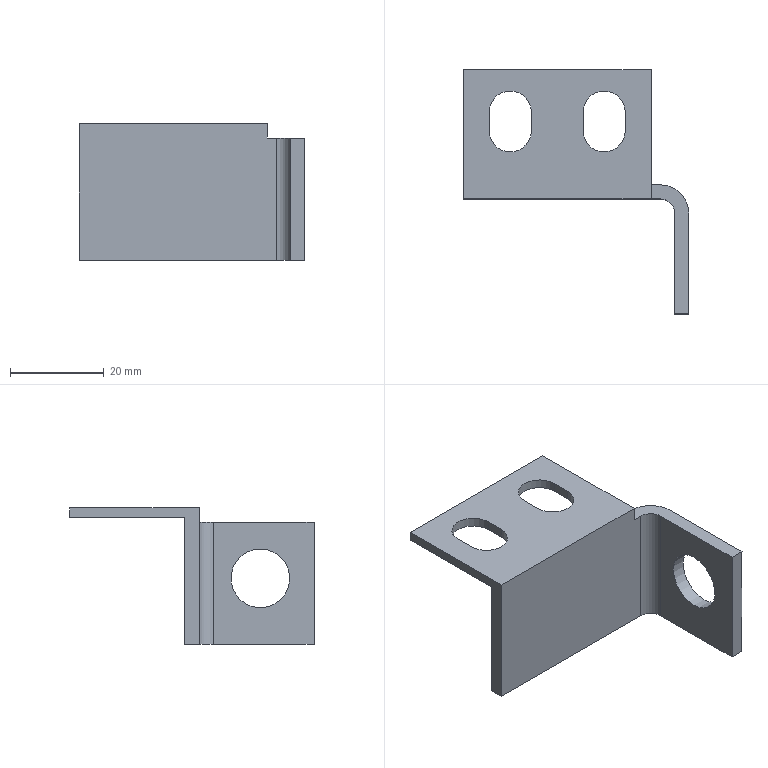Part | STEP file | lll_id4786_x_t | 1 solid | 23 faces | box 48 x 52 x 29 mm | volume 7058 mm3 | plane 16 | cylinder 7 | commonest cylinder face diameters 9 x4 6 x1 12 x1 12.5 x1
STEP:
#1=CARTESIAN_POINT('',(714.278,-390.043,-0.00000003));
#2=VERTEX_POINT('',#1);
#3=CARTESIAN_POINT('',(705.278,-390.043,-0.00000003));
#4=VERTEX_POINT('',#3);
#5=CARTESIAN_POINT('',(709.778,-390.043,-0.00000003));
#6=DIRECTION('',(0.,0.,1.));
#7=DIRECTION('',(1.,0.,0.));
#8=AXIS2_PLACEMENT_3D('',#5,#6,#7);
#9=CIRCLE('',#8,4.5);
#10=EDGE_CURVE('',#2,#4,#9,.T.);
#11=ORIENTED_EDGE('',*,*,#10,.T.);
#12=CARTESIAN_POINT('',(705.278,-394.043,-0.00000003));
#13=VERTEX_POINT('',#12);
#14=CARTESIAN_POINT('',(705.278,-392.043,-0.00000003));
#15=DIRECTION('',(0.,-1.,0.));
#16=VECTOR('',#15,1.);
#17=LINE('',#14,#16);
#18=EDGE_CURVE('',#4,#13,#17,.T.);
#19=ORIENTED_EDGE('',*,*,#18,.T.);
#20=CARTESIAN_POINT('',(714.278,-394.043,-0.00000003));
#21=VERTEX_POINT('',#20);
#22=CARTESIAN_POINT('',(709.778,-394.043,0.000000001));
#23=DIRECTION('',(0.,0.,-1.));
#24=DIRECTION('',(1.,0.,0.));
#25=AXIS2_PLACEMENT_3D('',#22,#23,#24);
#26=CIRCLE('',#25,4.5);
#27=EDGE_CURVE('',#21,#13,#26,.T.);
#28=ORIENTED_EDGE('',*,*,#27,.F.);
#29=CARTESIAN_POINT('',(714.278,-392.043,-0.00000003));
#30=DIRECTION('',(0.,1.,0.));
#31=VECTOR('',#30,1.);
#32=LINE('',#29,#31);
#33=EDGE_CURVE('',#21,#2,#32,.T.);
#34=ORIENTED_EDGE('',*,*,#33,.T.);
#35=EDGE_LOOP('',(#11,#19,#28,#34));
#36=FACE_BOUND('',#35,.T.);
#37=CARTESIAN_POINT('',(699.778,-405.543,0.000000001));
#38=VERTEX_POINT('',#37);
#39=CARTESIAN_POINT('',(739.778,-405.543,0.));
#40=VERTEX_POINT('',#39);
#41=CARTESIAN_POINT('',(758.537,-405.543,-0.000000001));
#42=DIRECTION('',(1.,0.,0.));
#43=VECTOR('',#42,1.);
#44=LINE('',#41,#43);
#45=EDGE_CURVE('',#38,#40,#44,.T.);
#46=ORIENTED_EDGE('',*,*,#45,.F.);
#47=CARTESIAN_POINT('',(699.778,-381.043,0.000000001));
#48=VERTEX_POINT('',#47);
#49=CARTESIAN_POINT('',(699.778,-172.043,0.000000001));
#50=DIRECTION('',(0.,1.,0.));
#51=VECTOR('',#50,1.);
#52=LINE('',#49,#51);
#53=EDGE_CURVE('',#38,#48,#52,.T.);
#54=ORIENTED_EDGE('',*,*,#53,.T.);
#55=CARTESIAN_POINT('',(739.778,-381.043,0.));
#56=VERTEX_POINT('',#55);
#57=CARTESIAN_POINT('',(1322.642,-381.043,-0.000000019));
#58=DIRECTION('',(1.,0.,0.));
#59=VECTOR('',#58,1.);
#60=LINE('',#57,#59);
#61=EDGE_CURVE('',#48,#56,#60,.T.);
#62=ORIENTED_EDGE('',*,*,#61,.T.);
#63=CARTESIAN_POINT('',(739.778,-397.043,0.));
#64=DIRECTION('',(0.,-1.,0.));
#65=VECTOR('',#64,1.);
#66=LINE('',#63,#65);
#67=EDGE_CURVE('',#56,#40,#66,.T.);
#68=ORIENTED_EDGE('',*,*,#67,.T.);
#69=EDGE_LOOP('',(#46,#54,#62,#68));
#70=FACE_BOUND('',#69,.T.);
#71=CARTESIAN_POINT('',(725.278,-390.043,-0.00000003));
#72=VERTEX_POINT('',#71);
#73=CARTESIAN_POINT('',(734.278,-390.043,-0.00000003));
#74=VERTEX_POINT('',#73);
#75=CARTESIAN_POINT('',(729.778,-390.043,-0.00000003));
#76=DIRECTION('',(0.,0.,-1.));
#77=DIRECTION('',(-1.,0.,0.));
#78=AXIS2_PLACEMENT_3D('',#75,#76,#77);
#79=CIRCLE('',#78,4.5);
#80=EDGE_CURVE('',#72,#74,#79,.T.);
#81=ORIENTED_EDGE('',*,*,#80,.F.);
#82=CARTESIAN_POINT('',(725.278,-394.043,-0.00000003));
#83=VERTEX_POINT('',#82);
#84=CARTESIAN_POINT('',(725.278,-392.043,-0.00000003));
#85=DIRECTION('',(0.,-1.,0.));
#86=VECTOR('',#85,1.);
#87=LINE('',#84,#86);
#88=EDGE_CURVE('',#72,#83,#87,.T.);
#89=ORIENTED_EDGE('',*,*,#88,.T.);
#90=CARTESIAN_POINT('',(734.278,-394.043,-0.00000003));
#91=VERTEX_POINT('',#90);
#92=CARTESIAN_POINT('',(729.778,-394.043,0.));
#93=DIRECTION('',(0.,0.,-1.));
#94=DIRECTION('',(-1.,0.,0.));
#95=AXIS2_PLACEMENT_3D('',#92,#93,#94);
#96=CIRCLE('',#95,4.5);
#97=EDGE_CURVE('',#91,#83,#96,.T.);
#98=ORIENTED_EDGE('',*,*,#97,.F.);
#99=CARTESIAN_POINT('',(734.278,-392.043,-0.00000003));
#100=DIRECTION('',(0.,1.,0.));
#101=VECTOR('',#100,1.);
#102=LINE('',#99,#101);
#103=EDGE_CURVE('',#91,#74,#102,.T.);
#104=ORIENTED_EDGE('',*,*,#103,.T.);
#105=EDGE_LOOP('',(#81,#89,#98,#104));
#106=FACE_BOUND('',#105,.T.);
#107=CARTESIAN_POINT('',(758.537,-172.043,-0.000000001));
#108=DIRECTION('',(0.,0.,-1.));
#109=DIRECTION('',(-1.,0.,0.));
#110=AXIS2_PLACEMENT_3D('',#107,#108,#109);
#111=PLANE('',#110);
#112=ADVANCED_FACE('',(#36,#70,#106),#111,.T.);
#113=CARTESIAN_POINT('',(739.778,-408.543,-1.));
#114=VERTEX_POINT('',#113);
#115=CARTESIAN_POINT('',(741.778,-408.543,-1.));
#116=VERTEX_POINT('',#115);
#117=CARTESIAN_POINT('',(712.778,-408.543,-1.));
#118=DIRECTION('',(1.,0.,0.));
#119=VECTOR('',#118,1.);
#120=LINE('',#117,#119);
#121=EDGE_CURVE('',#114,#116,#120,.T.);
#122=ORIENTED_EDGE('',*,*,#121,.F.);
#123=CARTESIAN_POINT('',(739.778,-408.543,2.));
#124=VERTEX_POINT('',#123);
#125=CARTESIAN_POINT('',(739.778,-408.543,-50.5));
#126=DIRECTION('',(0.,0.,1.));
#127=VECTOR('',#126,1.);
#128=LINE('',#125,#127);
#129=EDGE_CURVE('',#114,#124,#128,.T.);
#130=ORIENTED_EDGE('',*,*,#129,.T.);
#131=CARTESIAN_POINT('',(699.778,-408.543,2.));
#132=VERTEX_POINT('',#131);
#133=CARTESIAN_POINT('',(712.778,-408.543,2.));
#134=DIRECTION('',(1.,0.,0.));
#135=VECTOR('',#134,1.);
#136=LINE('',#133,#135);
#137=EDGE_CURVE('',#132,#124,#136,.T.);
#138=ORIENTED_EDGE('',*,*,#137,.F.);
#139=CARTESIAN_POINT('',(699.778,-408.543,-27.));
#140=VERTEX_POINT('',#139);
#141=CARTESIAN_POINT('',(699.778,-408.543,-50.5));
#142=DIRECTION('',(0.,0.,1.));
#143=VECTOR('',#142,1.);
#144=LINE('',#141,#143);
#145=EDGE_CURVE('',#140,#132,#144,.T.);
#146=ORIENTED_EDGE('',*,*,#145,.F.);
#147=CARTESIAN_POINT('',(741.778,-408.543,-27.));
#148=VERTEX_POINT('',#147);
#149=CARTESIAN_POINT('',(712.778,-408.543,-27.));
#150=DIRECTION('',(1.,0.,0.));
#151=VECTOR('',#150,1.);
#152=LINE('',#149,#151);
#153=EDGE_CURVE('',#140,#148,#152,.T.);
#154=ORIENTED_EDGE('',*,*,#153,.T.);
#155=CARTESIAN_POINT('',(741.778,-408.543,-55.5));
#156=DIRECTION('',(0.,0.,-1.));
#157=VECTOR('',#156,1.);
#158=LINE('',#155,#157);
#159=EDGE_CURVE('',#116,#148,#158,.T.);
#160=ORIENTED_EDGE('',*,*,#159,.F.);
#161=EDGE_LOOP('',(#122,#130,#138,#146,#154,#160));
#162=FACE_OUTER_BOUND('',#161,.T.);
#163=CARTESIAN_POINT('',(712.778,-408.543,-55.5));
#164=DIRECTION('',(0.,-1.,0.));
#165=DIRECTION('',(0.,0.,1.));
#166=AXIS2_PLACEMENT_3D('',#163,#164,#165);
#167=PLANE('',#166);
#168=ADVANCED_FACE('',(#162),#167,.T.);
#169=CARTESIAN_POINT('',(699.778,-405.543,-27.));
#170=VERTEX_POINT('',#169);
#171=CARTESIAN_POINT('',(741.778,-405.543,-27.));
#172=VERTEX_POINT('',#171);
#173=CARTESIAN_POINT('',(656.912,-405.543,-27.));
#174=DIRECTION('',(1.,0.,0.));
#175=VECTOR('',#174,1.);
#176=LINE('',#173,#175);
#177=EDGE_CURVE('',#170,#172,#176,.T.);
#178=ORIENTED_EDGE('',*,*,#177,.F.);
#179=CARTESIAN_POINT('',(699.778,-405.543,-33.));
#180=DIRECTION('',(0.,0.,1.));
#181=VECTOR('',#180,1.);
#182=LINE('',#179,#181);
#183=EDGE_CURVE('',#170,#38,#182,.T.);
#184=ORIENTED_EDGE('',*,*,#183,.T.);
#185=ORIENTED_EDGE('',*,*,#45,.T.);
#186=CARTESIAN_POINT('',(739.778,-405.543,-1.));
#187=VERTEX_POINT('',#186);
#188=CARTESIAN_POINT('',(739.778,-405.543,293.));
#189=DIRECTION('',(0.,0.,-1.));
#190=VECTOR('',#189,1.);
#191=LINE('',#188,#190);
#192=EDGE_CURVE('',#40,#187,#191,.T.);
#193=ORIENTED_EDGE('',*,*,#192,.T.);
#194=CARTESIAN_POINT('',(741.778,-405.543,-1.));
#195=VERTEX_POINT('',#194);
#196=CARTESIAN_POINT('',(1322.642,-405.543,-1.));
#197=DIRECTION('',(-1.,0.,0.));
#198=VECTOR('',#197,1.);
#199=LINE('',#196,#198);
#200=EDGE_CURVE('',#195,#187,#199,.T.);
#201=ORIENTED_EDGE('',*,*,#200,.F.);
#202=CARTESIAN_POINT('',(741.778,-405.543,288.));
#203=DIRECTION('',(0.,0.,1.));
#204=VECTOR('',#203,1.);
#205=LINE('',#202,#204);
#206=EDGE_CURVE('',#172,#195,#205,.T.);
#207=ORIENTED_EDGE('',*,*,#206,.F.);
#208=EDGE_LOOP('',(#178,#184,#185,#193,#201,#207));
#209=FACE_OUTER_BOUND('',#208,.T.);
#210=CARTESIAN_POINT('',(1322.642,-405.543,288.));
#211=DIRECTION('',(0.,-1.,0.));
#212=DIRECTION('',(0.,0.,1.));
#213=AXIS2_PLACEMENT_3D('',#210,#211,#212);
#214=PLANE('',#213);
#215=ADVANCED_FACE('',(#209),#214,.F.);
#216=CARTESIAN_POINT('',(747.778,-421.593,-19.25));
#217=VERTEX_POINT('',#216);
#218=CARTESIAN_POINT('',(747.778,-421.593,-13.));
#219=DIRECTION('',(1.,0.,0.));
#220=DIRECTION('',(0.,0.,-1.));
#221=AXIS2_PLACEMENT_3D('',#218,#219,#220);
#222=CIRCLE('',#221,6.25);
#223=EDGE_CURVE('',#217,#217,#222,.T.);
#224=ORIENTED_EDGE('',*,*,#223,.T.);
#225=EDGE_LOOP('',(#224));
#226=FACE_BOUND('',#225,.T.);
#227=CARTESIAN_POINT('',(744.778,-421.593,-19.25));
#228=VERTEX_POINT('',#227);
#229=CARTESIAN_POINT('',(744.778,-421.593,-13.));
#230=DIRECTION('',(1.,0.,0.));
#231=DIRECTION('',(0.,0.,-1.));
#232=AXIS2_PLACEMENT_3D('',#229,#230,#231);
#233=CIRCLE('',#232,6.25);
#234=EDGE_CURVE('',#228,#228,#233,.T.);
#235=ORIENTED_EDGE('',*,*,#234,.F.);
#236=EDGE_LOOP('',(#235));
#237=FACE_BOUND('',#236,.T.);
#238=CARTESIAN_POINT('',(751.33,-421.593,-13.));
#239=DIRECTION('',(-1.,0.,0.));
#240=DIRECTION('',(0.,0.,1.));
#241=AXIS2_PLACEMENT_3D('',#238,#239,#240);
#242=CYLINDRICAL_SURFACE('',#241,6.25);
#243=ADVANCED_FACE('',(#226,#237),#242,.F.);
#244=CARTESIAN_POINT('',(747.778,-433.043,-1.));
#245=VERTEX_POINT('',#244);
#246=CARTESIAN_POINT('',(747.778,-411.543,-1.));
#247=VERTEX_POINT('',#246);
#248=CARTESIAN_POINT('',(747.778,-400.043,-1.));
#249=DIRECTION('',(0.,1.,0.));
#250=VECTOR('',#249,1.);
#251=LINE('',#248,#250);
#252=EDGE_CURVE('',#245,#247,#251,.T.);
#253=ORIENTED_EDGE('',*,*,#252,.F.);
#254=CARTESIAN_POINT('',(747.778,-433.043,-27.));
#255=VERTEX_POINT('',#254);
#256=CARTESIAN_POINT('',(747.778,-433.043,-55.5));
#257=DIRECTION('',(0.,0.,1.));
#258=VECTOR('',#257,1.);
#259=LINE('',#256,#258);
#260=EDGE_CURVE('',#255,#245,#259,.T.);
#261=ORIENTED_EDGE('',*,*,#260,.F.);
#262=CARTESIAN_POINT('',(747.778,-411.543,-27.));
#263=VERTEX_POINT('',#262);
#264=CARTESIAN_POINT('',(747.778,-175.043,-27.));
#265=DIRECTION('',(0.,-1.,0.));
#266=VECTOR('',#265,1.);
#267=LINE('',#264,#266);
#268=EDGE_CURVE('',#263,#255,#267,.T.);
#269=ORIENTED_EDGE('',*,*,#268,.F.);
#270=CARTESIAN_POINT('',(747.778,-411.543,-55.5));
#271=DIRECTION('',(0.,0.,-1.));
#272=VECTOR('',#271,1.);
#273=LINE('',#270,#272);
#274=EDGE_CURVE('',#247,#263,#273,.T.);
#275=ORIENTED_EDGE('',*,*,#274,.F.);
#276=EDGE_LOOP('',(#253,#261,#269,#275));
#277=FACE_BOUND('',#276,.T.);
#278=ORIENTED_EDGE('',*,*,#223,.F.);
#279=EDGE_LOOP('',(#278));
#280=FACE_BOUND('',#279,.T.);
#281=CARTESIAN_POINT('',(747.778,-400.043,-55.5));
#282=DIRECTION('',(1.,0.,0.));
#283=DIRECTION('',(0.,0.,-1.));
#284=AXIS2_PLACEMENT_3D('',#281,#282,#283);
#285=PLANE('',#284);
#286=ADVANCED_FACE('',(#277,#280),#285,.T.);
#287=CARTESIAN_POINT('',(744.778,-433.043,-27.));
#288=VERTEX_POINT('',#287);
#289=CARTESIAN_POINT('',(744.778,-433.043,-1.));
#290=VERTEX_POINT('',#289);
#291=CARTESIAN_POINT('',(744.778,-433.043,-38.));
#292=DIRECTION('',(0.,0.,1.));
#293=VECTOR('',#292,1.);
#294=LINE('',#291,#293);
#295=EDGE_CURVE('',#288,#290,#294,.T.);
#296=ORIENTED_EDGE('',*,*,#295,.F.);
#297=CARTESIAN_POINT('',(759.128,-433.043,-27.));
#298=DIRECTION('',(1.,0.,0.));
#299=VECTOR('',#298,1.);
#300=LINE('',#297,#299);
#301=EDGE_CURVE('',#288,#255,#300,.T.);
#302=ORIENTED_EDGE('',*,*,#301,.T.);
#303=ORIENTED_EDGE('',*,*,#260,.T.);
#304=CARTESIAN_POINT('',(759.128,-433.043,-1.));
#305=DIRECTION('',(1.,0.,0.));
#306=VECTOR('',#305,1.);
#307=LINE('',#304,#306);
#308=EDGE_CURVE('',#290,#245,#307,.T.);
#309=ORIENTED_EDGE('',*,*,#308,.F.);
#310=EDGE_LOOP('',(#296,#302,#303,#309));
#311=FACE_OUTER_BOUND('',#310,.T.);
#312=CARTESIAN_POINT('',(759.128,-433.043,-22.));
#313=DIRECTION('',(0.,-1.,0.));
#314=DIRECTION('',(0.,0.,1.));
#315=AXIS2_PLACEMENT_3D('',#312,#313,#314);
#316=PLANE('',#315);
#317=ADVANCED_FACE('',(#311),#316,.T.);
#318=CARTESIAN_POINT('',(744.778,-411.543,-27.));
#319=VERTEX_POINT('',#318);
#320=CARTESIAN_POINT('',(744.778,-175.043,-27.));
#321=DIRECTION('',(0.,-1.,0.));
#322=VECTOR('',#321,1.);
#323=LINE('',#320,#322);
#324=EDGE_CURVE('',#319,#288,#323,.T.);
#325=ORIENTED_EDGE('',*,*,#324,.T.);
#326=ORIENTED_EDGE('',*,*,#295,.T.);
#327=CARTESIAN_POINT('',(744.778,-411.543,-1.));
#328=VERTEX_POINT('',#327);
#329=CARTESIAN_POINT('',(744.778,-401.543,-1.));
#330=DIRECTION('',(0.,1.,0.));
#331=VECTOR('',#330,1.);
#332=LINE('',#329,#331);
#333=EDGE_CURVE('',#290,#328,#332,.T.);
#334=ORIENTED_EDGE('',*,*,#333,.T.);
#335=CARTESIAN_POINT('',(744.778,-411.543,-38.));
#336=DIRECTION('',(0.,0.,1.));
#337=VECTOR('',#336,1.);
#338=LINE('',#335,#337);
#339=EDGE_CURVE('',#319,#328,#338,.T.);
#340=ORIENTED_EDGE('',*,*,#339,.F.);
#341=EDGE_LOOP('',(#325,#326,#334,#340));
#342=FACE_BOUND('',#341,.T.);
#343=ORIENTED_EDGE('',*,*,#234,.T.);
#344=EDGE_LOOP('',(#343));
#345=FACE_BOUND('',#344,.T.);
#346=CARTESIAN_POINT('',(744.778,-401.543,-38.));
#347=DIRECTION('',(1.,0.,0.));
#348=DIRECTION('',(0.,0.,-1.));
#349=AXIS2_PLACEMENT_3D('',#346,#347,#348);
#350=PLANE('',#349);
#351=ADVANCED_FACE('',(#342,#345),#350,.F.);
#352=CARTESIAN_POINT('',(741.778,-411.543,-1.));
#353=DIRECTION('',(0.,0.,1.));
#354=DIRECTION('',(-1.,0.,0.));
#355=AXIS2_PLACEMENT_3D('',#352,#353,#354);
#356=CIRCLE('',#355,3.);
#357=EDGE_CURVE('',#328,#116,#356,.T.);
#358=ORIENTED_EDGE('',*,*,#357,.T.);
#359=ORIENTED_EDGE('',*,*,#159,.T.);
#360=CARTESIAN_POINT('',(741.778,-411.543,-27.));
#361=DIRECTION('',(0.,0.,-1.));
#362=DIRECTION('',(-1.,0.,0.));
#363=AXIS2_PLACEMENT_3D('',#360,#361,#362);
#364=CIRCLE('',#363,3.);
#365=EDGE_CURVE('',#148,#319,#364,.T.);
#366=ORIENTED_EDGE('',*,*,#365,.T.);
#367=ORIENTED_EDGE('',*,*,#339,.T.);
#368=EDGE_LOOP('',(#358,#359,#366,#367));
#369=FACE_OUTER_BOUND('',#368,.T.);
#370=CARTESIAN_POINT('',(741.778,-411.543,-55.5));
#371=DIRECTION('',(0.,0.,-1.));
#372=DIRECTION('',(-1.,0.,0.));
#373=AXIS2_PLACEMENT_3D('',#370,#371,#372);
#374=CYLINDRICAL_SURFACE('',#373,3.);
#375=ADVANCED_FACE('',(#369),#374,.F.);
#376=ORIENTED_EDGE('',*,*,#153,.F.);
#377=CARTESIAN_POINT('',(699.778,-175.043,-27.));
#378=DIRECTION('',(0.,1.,0.));
#379=VECTOR('',#378,1.);
#380=LINE('',#377,#379);
#381=EDGE_CURVE('',#140,#170,#380,.T.);
#382=ORIENTED_EDGE('',*,*,#381,.T.);
#383=ORIENTED_EDGE('',*,*,#177,.T.);
#384=CARTESIAN_POINT('',(741.778,-411.543,-27.));
#385=DIRECTION('',(0.,0.,1.));
#386=DIRECTION('',(-1.,0.,0.));
#387=AXIS2_PLACEMENT_3D('',#384,#385,#386);
#388=CIRCLE('',#387,6.);
#389=EDGE_CURVE('',#263,#172,#388,.T.);
#390=ORIENTED_EDGE('',*,*,#389,.F.);
#391=ORIENTED_EDGE('',*,*,#268,.T.);
#392=ORIENTED_EDGE('',*,*,#301,.F.);
#393=ORIENTED_EDGE('',*,*,#324,.F.);
#394=ORIENTED_EDGE('',*,*,#365,.F.);
#395=EDGE_LOOP('',(#376,#382,#383,#390,#391,#392,#393,#394));
#396=FACE_OUTER_BOUND('',#395,.T.);
#397=CARTESIAN_POINT('',(656.912,-175.043,-27.));
#398=DIRECTION('',(0.,0.,1.));
#399=DIRECTION('',(1.,0.,0.));
#400=AXIS2_PLACEMENT_3D('',#397,#398,#399);
#401=PLANE('',#400);
#402=ADVANCED_FACE('',(#396),#401,.F.);
#403=ORIENTED_EDGE('',*,*,#389,.T.);
#404=ORIENTED_EDGE('',*,*,#206,.T.);
#405=CARTESIAN_POINT('',(741.778,-411.543,-1.));
#406=DIRECTION('',(0.,0.,-1.));
#407=DIRECTION('',(-1.,0.,0.));
#408=AXIS2_PLACEMENT_3D('',#405,#406,#407);
#409=CIRCLE('',#408,6.);
#410=EDGE_CURVE('',#195,#247,#409,.T.);
#411=ORIENTED_EDGE('',*,*,#410,.T.);
#412=ORIENTED_EDGE('',*,*,#274,.T.);
#413=EDGE_LOOP('',(#403,#404,#411,#412));
#414=FACE_OUTER_BOUND('',#413,.T.);
#415=CARTESIAN_POINT('',(741.778,-411.543,288.));
#416=DIRECTION('',(0.,0.,-1.));
#417=DIRECTION('',(-1.,0.,0.));
#418=AXIS2_PLACEMENT_3D('',#415,#416,#417);
#419=CYLINDRICAL_SURFACE('',#418,6.);
#420=ADVANCED_FACE('',(#414),#419,.T.);
#421=CARTESIAN_POINT('',(739.778,-332.043,-1.));
#422=DIRECTION('',(0.,1.,0.));
#423=VECTOR('',#422,1.);
#424=LINE('',#421,#423);
#425=EDGE_CURVE('',#114,#187,#424,.T.);
#426=ORIENTED_EDGE('',*,*,#425,.F.);
#427=ORIENTED_EDGE('',*,*,#121,.T.);
#428=ORIENTED_EDGE('',*,*,#357,.F.);
#429=ORIENTED_EDGE('',*,*,#333,.F.);
#430=ORIENTED_EDGE('',*,*,#308,.T.);
#431=ORIENTED_EDGE('',*,*,#252,.T.);
#432=ORIENTED_EDGE('',*,*,#410,.F.);
#433=ORIENTED_EDGE('',*,*,#200,.T.);
#434=EDGE_LOOP('',(#426,#427,#428,#429,#430,#431,#432,#433));
#435=FACE_OUTER_BOUND('',#434,.T.);
#436=CARTESIAN_POINT('',(768.128,-332.043,-1.));
#437=DIRECTION('',(0.,0.,1.));
#438=DIRECTION('',(-1.,0.,0.));
#439=AXIS2_PLACEMENT_3D('',#436,#437,#438);
#440=PLANE('',#439);
#441=ADVANCED_FACE('',(#435),#440,.T.);
#442=ORIENTED_EDGE('',*,*,#129,.F.);
#443=ORIENTED_EDGE('',*,*,#425,.T.);
#444=ORIENTED_EDGE('',*,*,#192,.F.);
#445=ORIENTED_EDGE('',*,*,#67,.F.);
#446=CARTESIAN_POINT('',(739.778,-381.043,2.));
#447=VERTEX_POINT('',#446);
#448=CARTESIAN_POINT('',(739.778,-381.043,321.));
#449=DIRECTION('',(0.,0.,1.));
#450=VECTOR('',#449,1.);
#451=LINE('',#448,#450);
#452=EDGE_CURVE('',#56,#447,#451,.T.);
#453=ORIENTED_EDGE('',*,*,#452,.T.);
#454=CARTESIAN_POINT('',(739.778,-329.043,2.));
#455=DIRECTION('',(0.,1.,0.));
#456=VECTOR('',#455,1.);
#457=LINE('',#454,#456);
#458=EDGE_CURVE('',#124,#447,#457,.T.);
#459=ORIENTED_EDGE('',*,*,#458,.F.);
#460=EDGE_LOOP('',(#442,#443,#444,#445,#453,#459));
#461=FACE_OUTER_BOUND('',#460,.T.);
#462=CARTESIAN_POINT('',(739.778,-392.543,3.));
#463=DIRECTION('',(1.,0.,0.));
#464=DIRECTION('',(0.,0.,-1.));
#465=AXIS2_PLACEMENT_3D('',#462,#463,#464);
#466=PLANE('',#465);
#467=ADVANCED_FACE('',(#461),#466,.T.);
#468=ORIENTED_EDGE('',*,*,#381,.F.);
#469=ORIENTED_EDGE('',*,*,#145,.T.);
#470=CARTESIAN_POINT('',(699.778,-381.043,2.));
#471=VERTEX_POINT('',#470);
#472=CARTESIAN_POINT('',(699.778,-74.611,2.));
#473=DIRECTION('',(0.,-1.,0.));
#474=VECTOR('',#473,1.);
#475=LINE('',#472,#474);
#476=EDGE_CURVE('',#471,#132,#475,.T.);
#477=ORIENTED_EDGE('',*,*,#476,.F.);
#478=CARTESIAN_POINT('',(699.778,-381.043,321.));
#479=DIRECTION('',(0.,0.,1.));
#480=VECTOR('',#479,1.);
#481=LINE('',#478,#480);
#482=EDGE_CURVE('',#48,#471,#481,.T.);
#483=ORIENTED_EDGE('',*,*,#482,.F.);
#484=ORIENTED_EDGE('',*,*,#53,.F.);
#485=ORIENTED_EDGE('',*,*,#183,.F.);
#486=EDGE_LOOP('',(#468,#469,#477,#483,#484,#485));
#487=FACE_OUTER_BOUND('',#486,.T.);
#488=CARTESIAN_POINT('',(699.778,-74.611,-33.));
#489=DIRECTION('',(1.,0.,0.));
#490=DIRECTION('',(0.,0.,-1.));
#491=AXIS2_PLACEMENT_3D('',#488,#489,#490);
#492=PLANE('',#491);
#493=ADVANCED_FACE('',(#487),#492,.F.);
#494=CARTESIAN_POINT('',(705.278,-394.043,2.));
#495=VERTEX_POINT('',#494);
#496=CARTESIAN_POINT('',(705.278,-394.043,1280.));
#497=DIRECTION('',(0.,0.,-1.));
#498=VECTOR('',#497,1.);
#499=LINE('',#496,#498);
#500=EDGE_CURVE('',#495,#13,#499,.T.);
#501=ORIENTED_EDGE('',*,*,#500,.F.);
#502=CARTESIAN_POINT('',(714.278,-394.043,2.));
#503=VERTEX_POINT('',#502);
#504=CARTESIAN_POINT('',(709.778,-394.043,2.));
#505=DIRECTION('',(0.,0.,-1.));
#506=DIRECTION('',(-1.,0.,0.));
#507=AXIS2_PLACEMENT_3D('',#504,#505,#506);
#508=CIRCLE('',#507,4.5);
#509=EDGE_CURVE('',#503,#495,#508,.T.);
#510=ORIENTED_EDGE('',*,*,#509,.F.);
#511=CARTESIAN_POINT('',(714.278,-394.043,1280.));
#512=DIRECTION('',(0.,0.,1.));
#513=VECTOR('',#512,1.);
#514=LINE('',#511,#513);
#515=EDGE_CURVE('',#21,#503,#514,.T.);
#516=ORIENTED_EDGE('',*,*,#515,.F.);
#517=ORIENTED_EDGE('',*,*,#27,.T.);
#518=EDGE_LOOP('',(#501,#510,#516,#517));
#519=FACE_OUTER_BOUND('',#518,.T.);
#520=CARTESIAN_POINT('',(709.778,-394.043,50.));
#521=DIRECTION('',(0.,0.,-1.));
#522=DIRECTION('',(-1.,0.,0.));
#523=AXIS2_PLACEMENT_3D('',#520,#521,#522);
#524=CYLINDRICAL_SURFACE('',#523,4.5);
#525=ADVANCED_FACE('',(#519),#524,.F.);
#526=CARTESIAN_POINT('',(725.278,-394.043,2.));
#527=VERTEX_POINT('',#526);
#528=CARTESIAN_POINT('',(725.278,-394.043,1280.));
#529=DIRECTION('',(0.,0.,-1.));
#530=VECTOR('',#529,1.);
#531=LINE('',#528,#530);
#532=EDGE_CURVE('',#527,#83,#531,.T.);
#533=ORIENTED_EDGE('',*,*,#532,.F.);
#534=CARTESIAN_POINT('',(734.278,-394.043,2.));
#535=VERTEX_POINT('',#534);
#536=CARTESIAN_POINT('',(729.778,-394.043,2.));
#537=DIRECTION('',(0.,0.,-1.));
#538=DIRECTION('',(-1.,0.,0.));
#539=AXIS2_PLACEMENT_3D('',#536,#537,#538);
#540=CIRCLE('',#539,4.5);
#541=EDGE_CURVE('',#535,#527,#540,.T.);
#542=ORIENTED_EDGE('',*,*,#541,.F.);
#543=CARTESIAN_POINT('',(734.278,-394.043,1280.));
#544=DIRECTION('',(0.,0.,1.));
#545=VECTOR('',#544,1.);
#546=LINE('',#543,#545);
#547=EDGE_CURVE('',#91,#535,#546,.T.);
#548=ORIENTED_EDGE('',*,*,#547,.F.);
#549=ORIENTED_EDGE('',*,*,#97,.T.);
#550=EDGE_LOOP('',(#533,#542,#548,#549));
#551=FACE_OUTER_BOUND('',#550,.T.);
#552=CARTESIAN_POINT('',(729.778,-394.043,50.));
#553=DIRECTION('',(0.,0.,-1.));
#554=DIRECTION('',(1.,0.,0.));
#555=AXIS2_PLACEMENT_3D('',#552,#553,#554);
#556=CYLINDRICAL_SURFACE('',#555,4.5);
#557=ADVANCED_FACE('',(#551),#556,.F.);
#558=ORIENTED_EDGE('',*,*,#482,.T.);
#559=CARTESIAN_POINT('',(768.128,-381.043,2.));
#560=DIRECTION('',(1.,0.,0.));
#561=VECTOR('',#560,1.);
#562=LINE('',#559,#561);
#563=EDGE_CURVE('',#471,#447,#562,.T.);
#564=ORIENTED_EDGE('',*,*,#563,.T.);
#565=ORIENTED_EDGE('',*,*,#452,.F.);
#566=ORIENTED_EDGE('',*,*,#61,.F.);
#567=EDGE_LOOP('',(#558,#564,#565,#566));
#568=FACE_OUTER_BOUND('',#567,.T.);
#569=CARTESIAN_POINT('',(1322.642,-381.043,321.));
#570=DIRECTION('',(0.,-1.,0.));
#571=DIRECTION('',(0.,0.,1.));
#572=AXIS2_PLACEMENT_3D('',#569,#570,#571);
#573=PLANE('',#572);
#574=ADVANCED_FACE('',(#568),#573,.F.);
#575=CARTESIAN_POINT('',(725.278,-390.043,2.));
#576=VERTEX_POINT('',#575);
#577=CARTESIAN_POINT('',(725.278,-329.043,2.));
#578=DIRECTION('',(0.,-1.,0.));
#579=VECTOR('',#578,1.);
#580=LINE('',#577,#579);
#581=EDGE_CURVE('',#576,#527,#580,.T.);
#582=ORIENTED_EDGE('',*,*,#581,.F.);
#583=CARTESIAN_POINT('',(734.278,-390.043,2.));
#584=VERTEX_POINT('',#583);
#585=CARTESIAN_POINT('',(729.778,-390.043,2.));
#586=DIRECTION('',(0.,0.,1.));
#587=DIRECTION('',(1.,0.,0.));
#588=AXIS2_PLACEMENT_3D('',#585,#586,#587);
#589=CIRCLE('',#588,4.5);
#590=EDGE_CURVE('',#584,#576,#589,.T.);
#591=ORIENTED_EDGE('',*,*,#590,.F.);
#592=CARTESIAN_POINT('',(734.278,-329.043,2.));
#593=DIRECTION('',(0.,1.,0.));
#594=VECTOR('',#593,1.);
#595=LINE('',#592,#594);
#596=EDGE_CURVE('',#535,#584,#595,.T.);
#597=ORIENTED_EDGE('',*,*,#596,.F.);
#598=ORIENTED_EDGE('',*,*,#541,.T.);
#599=EDGE_LOOP('',(#582,#591,#597,#598));
#600=FACE_BOUND('',#599,.T.);
#601=CARTESIAN_POINT('',(705.278,-390.043,2.));
#602=VERTEX_POINT('',#601);
#603=CARTESIAN_POINT('',(705.278,-329.043,2.));
#604=DIRECTION('',(0.,-1.,0.));
#605=VECTOR('',#604,1.);
#606=LINE('',#603,#605);
#607=EDGE_CURVE('',#602,#495,#606,.T.);
#608=ORIENTED_EDGE('',*,*,#607,.F.);
#609=CARTESIAN_POINT('',(714.278,-390.043,2.));
#610=VERTEX_POINT('',#609);
#611=CARTESIAN_POINT('',(709.778,-390.043,2.));
#612=DIRECTION('',(0.,0.,-1.));
#613=DIRECTION('',(1.,0.,0.));
#614=AXIS2_PLACEMENT_3D('',#611,#612,#613);
#615=CIRCLE('',#614,4.5);
#616=EDGE_CURVE('',#602,#610,#615,.T.);
#617=ORIENTED_EDGE('',*,*,#616,.T.);
#618=CARTESIAN_POINT('',(714.278,-329.043,2.));
#619=DIRECTION('',(0.,1.,0.));
#620=VECTOR('',#619,1.);
#621=LINE('',#618,#620);
#622=EDGE_CURVE('',#503,#610,#621,.T.);
#623=ORIENTED_EDGE('',*,*,#622,.F.);
#624=ORIENTED_EDGE('',*,*,#509,.T.);
#625=EDGE_LOOP('',(#608,#617,#623,#624));
#626=FACE_BOUND('',#625,.T.);
#627=ORIENTED_EDGE('',*,*,#137,.T.);
#628=ORIENTED_EDGE('',*,*,#458,.T.);
#629=ORIENTED_EDGE('',*,*,#563,.F.);
#630=ORIENTED_EDGE('',*,*,#476,.T.);
#631=EDGE_LOOP('',(#627,#628,#629,#630));
#632=FACE_BOUND('',#631,.T.);
#633=CARTESIAN_POINT('',(768.128,-329.043,2.));
#634=DIRECTION('',(0.,0.,1.));
#635=DIRECTION('',(-1.,0.,0.));
#636=AXIS2_PLACEMENT_3D('',#633,#634,#635);
#637=PLANE('',#636);
#638=ADVANCED_FACE('',(#600,#626,#632),#637,.T.);
#639=ORIENTED_EDGE('',*,*,#607,.T.);
#640=ORIENTED_EDGE('',*,*,#500,.T.);
#641=ORIENTED_EDGE('',*,*,#18,.F.);
#642=CARTESIAN_POINT('',(705.278,-390.043,-0.00000003));
#643=DIRECTION('',(0.,0.,-1.));
#644=VECTOR('',#643,1.);
#645=LINE('',#642,#644);
#646=EDGE_CURVE('',#602,#4,#645,.T.);
#647=ORIENTED_EDGE('',*,*,#646,.F.);
#648=EDGE_LOOP('',(#639,#640,#641,#647));
#649=FACE_OUTER_BOUND('',#648,.T.);
#650=CARTESIAN_POINT('',(705.278,-392.043,-0.00000003));
#651=DIRECTION('',(-1.,0.,0.));
#652=DIRECTION('',(0.,0.,1.));
#653=AXIS2_PLACEMENT_3D('',#650,#651,#652);
#654=PLANE('',#653);
#655=ADVANCED_FACE('',(#649),#654,.F.);
#656=ORIENTED_EDGE('',*,*,#622,.T.);
#657=CARTESIAN_POINT('',(714.278,-390.043,-0.00000003));
#658=DIRECTION('',(0.,0.,-1.));
#659=VECTOR('',#658,1.);
#660=LINE('',#657,#659);
#661=EDGE_CURVE('',#610,#2,#660,.T.);
#662=ORIENTED_EDGE('',*,*,#661,.T.);
#663=ORIENTED_EDGE('',*,*,#33,.F.);
#664=ORIENTED_EDGE('',*,*,#515,.T.);
#665=EDGE_LOOP('',(#656,#662,#663,#664));
#666=FACE_OUTER_BOUND('',#665,.T.);
#667=CARTESIAN_POINT('',(714.278,-392.043,-0.00000003));
#668=DIRECTION('',(1.,0.,0.));
#669=DIRECTION('',(0.,0.,-1.));
#670=AXIS2_PLACEMENT_3D('',#667,#668,#669);
#671=PLANE('',#670);
#672=ADVANCED_FACE('',(#666),#671,.F.);
#673=ORIENTED_EDGE('',*,*,#646,.T.);
#674=ORIENTED_EDGE('',*,*,#10,.F.);
#675=ORIENTED_EDGE('',*,*,#661,.F.);
#676=ORIENTED_EDGE('',*,*,#616,.F.);
#677=EDGE_LOOP('',(#673,#674,#675,#676));
#678=FACE_OUTER_BOUND('',#677,.T.);
#679=CARTESIAN_POINT('',(709.778,-390.043,1280.));
#680=DIRECTION('',(0.,0.,-1.));
#681=DIRECTION('',(-1.,0.,0.));
#682=AXIS2_PLACEMENT_3D('',#679,#680,#681);
#683=CYLINDRICAL_SURFACE('',#682,4.5);
#684=ADVANCED_FACE('',(#678),#683,.F.);
#685=ORIENTED_EDGE('',*,*,#581,.T.);
#686=ORIENTED_EDGE('',*,*,#532,.T.);
#687=ORIENTED_EDGE('',*,*,#88,.F.);
#688=CARTESIAN_POINT('',(725.278,-390.043,-0.00000003));
#689=DIRECTION('',(0.,0.,-1.));
#690=VECTOR('',#689,1.);
#691=LINE('',#688,#690);
#692=EDGE_CURVE('',#576,#72,#691,.T.);
#693=ORIENTED_EDGE('',*,*,#692,.F.);
#694=EDGE_LOOP('',(#685,#686,#687,#693));
#695=FACE_OUTER_BOUND('',#694,.T.);
#696=CARTESIAN_POINT('',(725.278,-392.043,-0.00000003));
#697=DIRECTION('',(-1.,0.,0.));
#698=DIRECTION('',(0.,0.,1.));
#699=AXIS2_PLACEMENT_3D('',#696,#697,#698);
#700=PLANE('',#699);
#701=ADVANCED_FACE('',(#695),#700,.F.);
#702=ORIENTED_EDGE('',*,*,#596,.T.);
#703=CARTESIAN_POINT('',(734.278,-390.043,-0.00000003));
#704=DIRECTION('',(0.,0.,-1.));
#705=VECTOR('',#704,1.);
#706=LINE('',#703,#705);
#707=EDGE_CURVE('',#584,#74,#706,.T.);
#708=ORIENTED_EDGE('',*,*,#707,.T.);
#709=ORIENTED_EDGE('',*,*,#103,.F.);
#710=ORIENTED_EDGE('',*,*,#547,.T.);
#711=EDGE_LOOP('',(#702,#708,#709,#710));
#712=FACE_OUTER_BOUND('',#711,.T.);
#713=CARTESIAN_POINT('',(734.278,-392.043,-0.00000003));
#714=DIRECTION('',(1.,0.,0.));
#715=DIRECTION('',(0.,0.,-1.));
#716=AXIS2_PLACEMENT_3D('',#713,#714,#715);
#717=PLANE('',#716);
#718=ADVANCED_FACE('',(#712),#717,.F.);
#719=ORIENTED_EDGE('',*,*,#590,.T.);
#720=ORIENTED_EDGE('',*,*,#692,.T.);
#721=ORIENTED_EDGE('',*,*,#80,.T.);
#722=ORIENTED_EDGE('',*,*,#707,.F.);
#723=EDGE_LOOP('',(#719,#720,#721,#722));
#724=FACE_OUTER_BOUND('',#723,.T.);
#725=CARTESIAN_POINT('',(729.778,-390.043,1280.));
#726=DIRECTION('',(0.,0.,-1.));
#727=DIRECTION('',(-1.,0.,0.));
#728=AXIS2_PLACEMENT_3D('',#725,#726,#727);
#729=CYLINDRICAL_SURFACE('',#728,4.5);
#730=ADVANCED_FACE('',(#724),#729,.F.);
#731=CLOSED_SHELL('',(#112,#168,#215,#243,#286,#317,#351,#375,#402,#420,#441,#467,#493,#525,#557,#574,#638,#655,#672,#684,#701,#718,#730));
#732=MANIFOLD_SOLID_BREP('',#731);
#733=(LENGTH_UNIT()NAMED_UNIT(*)SI_UNIT(.MILLI.,.METRE.));
#734=UNCERTAINTY_MEASURE_WITH_UNIT(LENGTH_MEASURE(0.00002),#733,'','');
#735=(NAMED_UNIT(*)PLANE_ANGLE_UNIT()SI_UNIT($,.RADIAN.));
#736=PLANE_ANGLE_MEASURE_WITH_UNIT(PLANE_ANGLE_MEASURE(0.01745),#735);
#737=DIMENSIONAL_EXPONENTS(0.,0.,0.,0.,0.,0.,0.);
#738=(CONVERSION_BASED_UNIT('DEGREE',#736)NAMED_UNIT(#737)PLANE_ANGLE_UNIT());
#739=(NAMED_UNIT(*)SI_UNIT($,.STERADIAN.)SOLID_ANGLE_UNIT());
#740=(GEOMETRIC_REPRESENTATION_CONTEXT(3)GLOBAL_UNCERTAINTY_ASSIGNED_CONTEXT((#734))GLOBAL_UNIT_ASSIGNED_CONTEXT((#733,#738,#739))REPRESENTATION_CONTEXT('',''));
#741=ADVANCED_BREP_SHAPE_REPRESENTATION('',(#732),#740);